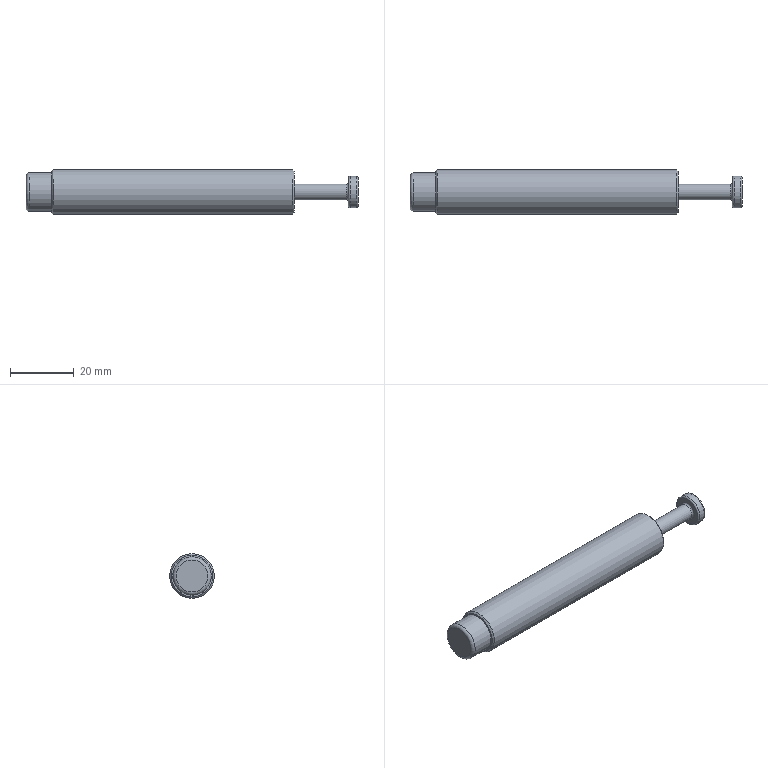Part | STEP file | Tube feed_id454_x_t | 1 solid | 15 faces | box 104 x 14 x 14 mm | volume 13153 mm3 | plane 5 | cylinder 4 | torus 4 | cone 2 | commonest cylinder face diameters 5 x1 10 x1 12 x1 14 x1
STEP:
#1=CARTESIAN_POINT('',(0.,0.,0.));
#2=DIRECTION('',(0.,0.,1.));
#3=DIRECTION('',(1.,0.,0.));
#4=AXIS2_PLACEMENT_3D('',#1,#2,#3);
#5=CARTESIAN_POINT('',(-13.,376.936,-66.));
#6=VERTEX_POINT('',#5);
#7=CARTESIAN_POINT('',(-13.,376.936,-72.));
#8=DIRECTION('',(1.,0.,0.));
#9=DIRECTION('',(0.,0.,1.));
#10=AXIS2_PLACEMENT_3D('',#7,#8,#9);
#11=CIRCLE('',#10,6.);
#12=CARTESIAN_POINT('',(-14.,376.936,-72.));
#13=DIRECTION('',(1.,0.,0.));
#14=DIRECTION('',(0.,0.,-1.));
#15=AXIS2_PLACEMENT_3D('',#12,#13,#14);
#16=CYLINDRICAL_SURFACE('',#15,6.);
#17=CARTESIAN_POINT('',(3.142,1.));
#18=DIRECTION('',(1.,0.));
#19=VECTOR('',#18,1.);
#20=LINE('',#17,#19);
#21=(GEOMETRIC_REPRESENTATION_CONTEXT(2)PARAMETRIC_REPRESENTATION_CONTEXT()REPRESENTATION_CONTEXT('',''));
#22=DEFINITIONAL_REPRESENTATION('',(#20),#21);
#23=PCURVE('',#16,#22);
#24=CARTESIAN_POINT('',(-13.,376.936,-72.));
#25=DIRECTION('',(-1.,0.,0.));
#26=DIRECTION('',(0.,0.,1.));
#27=AXIS2_PLACEMENT_3D('',#24,#25,#26);
#28=TOROIDAL_SURFACE('',#27,5.,1.);
#29=CARTESIAN_POINT('',(6.283,6.283));
#30=DIRECTION('',(-1.,0.));
#31=VECTOR('',#30,1.);
#32=LINE('',#29,#31);
#33=(GEOMETRIC_REPRESENTATION_CONTEXT(2)PARAMETRIC_REPRESENTATION_CONTEXT()REPRESENTATION_CONTEXT('',''));
#34=DEFINITIONAL_REPRESENTATION('',(#32),#33);
#35=PCURVE('',#28,#34);
#36=SURFACE_CURVE('',#11,(#23,#35),.PCURVE_S1.);
#37=EDGE_CURVE('',#6,#6,#36,.T.);
#38=ORIENTED_EDGE('',*,*,#37,.T.);
#39=CARTESIAN_POINT('',(-6.,376.936,-66.));
#40=VERTEX_POINT('',#39);
#41=CARTESIAN_POINT('',(-13.,376.936,-66.));
#42=CARTESIAN_POINT('',(-6.,376.936,-66.));
#43=B_SPLINE_CURVE_WITH_KNOTS('',1,(#41,#42),.UNSPECIFIED.,.F.,.F.,(2,2),(1.,8.),.PIECEWISE_BEZIER_KNOTS.);
#44=CARTESIAN_POINT('',(9.425,0.));
#45=DIRECTION('',(0.,1.));
#46=VECTOR('',#45,1.);
#47=LINE('',#44,#46);
#48=(GEOMETRIC_REPRESENTATION_CONTEXT(2)PARAMETRIC_REPRESENTATION_CONTEXT()REPRESENTATION_CONTEXT('',''));
#49=DEFINITIONAL_REPRESENTATION('',(#47),#48);
#50=PCURVE('',#16,#49);
#51=CARTESIAN_POINT('',(3.142,0.));
#52=DIRECTION('',(0.,1.));
#53=VECTOR('',#52,1.);
#54=LINE('',#51,#53);
#55=(GEOMETRIC_REPRESENTATION_CONTEXT(2)PARAMETRIC_REPRESENTATION_CONTEXT()REPRESENTATION_CONTEXT('',''));
#56=DEFINITIONAL_REPRESENTATION('',(#54),#55);
#57=PCURVE('',#16,#56);
#58=SEAM_CURVE('',#43,(#50,#57),.PCURVE_S1.);
#59=EDGE_CURVE('',#6,#40,#58,.T.);
#60=ORIENTED_EDGE('',*,*,#59,.T.);
#61=CARTESIAN_POINT('',(-6.,376.936,-72.));
#62=DIRECTION('',(-1.,0.,0.));
#63=DIRECTION('',(0.,0.,1.));
#64=AXIS2_PLACEMENT_3D('',#61,#62,#63);
#65=CIRCLE('',#64,6.);
#66=CARTESIAN_POINT('',(9.425,8.));
#67=DIRECTION('',(-1.,0.));
#68=VECTOR('',#67,1.);
#69=LINE('',#66,#68);
#70=(GEOMETRIC_REPRESENTATION_CONTEXT(2)PARAMETRIC_REPRESENTATION_CONTEXT()REPRESENTATION_CONTEXT('',''));
#71=DEFINITIONAL_REPRESENTATION('',(#69),#70);
#72=PCURVE('',#16,#71);
#73=CARTESIAN_POINT('',(-6.,376.936,-72.));
#74=DIRECTION('',(-1.,0.,0.));
#75=DIRECTION('',(0.,0.,1.));
#76=AXIS2_PLACEMENT_3D('',#73,#74,#75);
#77=PLANE('',#76);
#78=CARTESIAN_POINT('',(0.,0.));
#79=DIRECTION('',(1.,0.));
#80=AXIS2_PLACEMENT_2D('',#78,#79);
#81=CIRCLE('',#80,6.);
#82=(GEOMETRIC_REPRESENTATION_CONTEXT(2)PARAMETRIC_REPRESENTATION_CONTEXT()REPRESENTATION_CONTEXT('',''));
#83=DEFINITIONAL_REPRESENTATION('',(#81),#82);
#84=PCURVE('',#77,#83);
#85=SURFACE_CURVE('',#65,(#72,#84),.PCURVE_S1.);
#86=EDGE_CURVE('',#40,#40,#85,.T.);
#87=ORIENTED_EDGE('',*,*,#86,.T.);
#88=ORIENTED_EDGE('',*,*,#59,.F.);
#89=EDGE_LOOP('',(#38,#60,#87,#88));
#90=FACE_BOUND('',#89,.T.);
#91=ADVANCED_FACE('',(#90),#16,.T.);
#92=CARTESIAN_POINT('',(-14.,376.936,-67.));
#93=VERTEX_POINT('',#92);
#94=CARTESIAN_POINT('',(-14.,376.936,-72.));
#95=DIRECTION('',(-1.,0.,0.));
#96=DIRECTION('',(0.,0.,1.));
#97=AXIS2_PLACEMENT_3D('',#94,#95,#96);
#98=CIRCLE('',#97,5.);
#99=CARTESIAN_POINT('',(-14.,376.936,-72.));
#100=DIRECTION('',(-1.,0.,0.));
#101=DIRECTION('',(0.,0.,1.));
#102=AXIS2_PLACEMENT_3D('',#99,#100,#101);
#103=PLANE('',#102);
#104=CARTESIAN_POINT('',(0.,0.));
#105=DIRECTION('',(1.,0.));
#106=AXIS2_PLACEMENT_2D('',#104,#105);
#107=CIRCLE('',#106,5.);
#108=(GEOMETRIC_REPRESENTATION_CONTEXT(2)PARAMETRIC_REPRESENTATION_CONTEXT()REPRESENTATION_CONTEXT('',''));
#109=DEFINITIONAL_REPRESENTATION('',(#107),#108);
#110=PCURVE('',#103,#109);
#111=CARTESIAN_POINT('',(0.,7.854));
#112=DIRECTION('',(1.,0.));
#113=VECTOR('',#112,1.);
#114=LINE('',#111,#113);
#115=(GEOMETRIC_REPRESENTATION_CONTEXT(2)PARAMETRIC_REPRESENTATION_CONTEXT()REPRESENTATION_CONTEXT('',''));
#116=DEFINITIONAL_REPRESENTATION('',(#114),#115);
#117=PCURVE('',#28,#116);
#118=SURFACE_CURVE('',#98,(#110,#117),.PCURVE_S1.);
#119=EDGE_CURVE('',#93,#93,#118,.T.);
#120=ORIENTED_EDGE('',*,*,#119,.T.);
#121=EDGE_LOOP('',(#120));
#122=FACE_BOUND('',#121,.T.);
#123=ADVANCED_FACE('',(#122),#103,.T.);
#124=CARTESIAN_POINT('',(-6.,376.936,-65.5));
#125=VERTEX_POINT('',#124);
#126=CARTESIAN_POINT('',(-6.,376.936,-72.));
#127=DIRECTION('',(-1.,0.,0.));
#128=DIRECTION('',(0.,0.,1.));
#129=AXIS2_PLACEMENT_3D('',#126,#127,#128);
#130=CIRCLE('',#129,6.5);
#131=CARTESIAN_POINT('',(0.,0.));
#132=DIRECTION('',(1.,0.));
#133=AXIS2_PLACEMENT_2D('',#131,#132);
#134=CIRCLE('',#133,6.5);
#135=(GEOMETRIC_REPRESENTATION_CONTEXT(2)PARAMETRIC_REPRESENTATION_CONTEXT()REPRESENTATION_CONTEXT('',''));
#136=DEFINITIONAL_REPRESENTATION('',(#134),#135);
#137=PCURVE('',#77,#136);
#138=CARTESIAN_POINT('',(-5.5,376.936,-72.));
#139=DIRECTION('',(1.,0.,0.));
#140=DIRECTION('',(0.,0.,-1.));
#141=AXIS2_PLACEMENT_3D('',#138,#139,#140);
#142=CONICAL_SURFACE('',#141,7.,0.7854);
#143=CARTESIAN_POINT('',(9.425,-0.5));
#144=DIRECTION('',(-1.,0.));
#145=VECTOR('',#144,1.);
#146=LINE('',#143,#145);
#147=(GEOMETRIC_REPRESENTATION_CONTEXT(2)PARAMETRIC_REPRESENTATION_CONTEXT()REPRESENTATION_CONTEXT('',''));
#148=DEFINITIONAL_REPRESENTATION('',(#146),#147);
#149=PCURVE('',#142,#148);
#150=SURFACE_CURVE('',#130,(#137,#149),.PCURVE_S1.);
#151=EDGE_CURVE('',#125,#125,#150,.T.);
#152=ORIENTED_EDGE('',*,*,#151,.T.);
#153=EDGE_LOOP('',(#152));
#154=FACE_BOUND('',#153,.T.);
#155=ORIENTED_EDGE('',*,*,#86,.F.);
#156=EDGE_LOOP('',(#155));
#157=FACE_BOUND('',#156,.T.);
#158=ADVANCED_FACE('',(#154,#157),#77,.T.);
#159=CARTESIAN_POINT('',(70.,376.936,-74.5));
#160=VERTEX_POINT('',#159);
#161=CARTESIAN_POINT('',(70.,376.936,-72.));
#162=DIRECTION('',(1.,0.,0.));
#163=DIRECTION('',(0.,0.,-1.));
#164=AXIS2_PLACEMENT_3D('',#161,#162,#163);
#165=CIRCLE('',#164,2.5);
#166=CARTESIAN_POINT('',(70.,376.936,-72.));
#167=DIRECTION('',(-1.,0.,0.));
#168=DIRECTION('',(0.,0.,1.));
#169=AXIS2_PLACEMENT_3D('',#166,#167,#168);
#170=PLANE('',#169);
#171=CARTESIAN_POINT('',(-2.5,0.));
#172=CARTESIAN_POINT('',(-2.5,4.33));
#173=CARTESIAN_POINT('',(1.25,2.165));
#174=CARTESIAN_POINT('',(5.,0.));
#175=CARTESIAN_POINT('',(1.25,-2.165));
#176=CARTESIAN_POINT('',(-2.5,-4.33));
#177=CARTESIAN_POINT('',(-2.5,0.));
#178=(BOUNDED_CURVE()B_SPLINE_CURVE(2,(#171,#172,#173,#174,#175,#176,#177),.UNSPECIFIED.,.T.,.F.)B_SPLINE_CURVE_WITH_KNOTS((1,2,2,2,2,1),(-2.094,0.,2.094,4.189,6.283,8.378),.UNSPECIFIED.)CURVE()GEOMETRIC_REPRESENTATION_ITEM()RATIONAL_B_SPLINE_CURVE((1.,0.5,1.,0.5,1.,0.5,1.))REPRESENTATION_ITEM(''));
#179=(GEOMETRIC_REPRESENTATION_CONTEXT(2)PARAMETRIC_REPRESENTATION_CONTEXT()REPRESENTATION_CONTEXT('',''));
#180=DEFINITIONAL_REPRESENTATION('',(#178),#179);
#181=PCURVE('',#170,#180);
#182=CARTESIAN_POINT('',(90.,376.936,-72.));
#183=DIRECTION('',(-1.,0.,0.));
#184=DIRECTION('',(0.,0.,1.));
#185=AXIS2_PLACEMENT_3D('',#182,#183,#184);
#186=CYLINDRICAL_SURFACE('',#185,2.5);
#187=CARTESIAN_POINT('',(9.425,20.));
#188=DIRECTION('',(-1.,0.));
#189=VECTOR('',#188,1.);
#190=LINE('',#187,#189);
#191=(GEOMETRIC_REPRESENTATION_CONTEXT(2)PARAMETRIC_REPRESENTATION_CONTEXT()REPRESENTATION_CONTEXT('',''));
#192=DEFINITIONAL_REPRESENTATION('',(#190),#191);
#193=PCURVE('',#186,#192);
#194=SURFACE_CURVE('',#165,(#181,#193),.PCURVE_S1.);
#195=EDGE_CURVE('',#160,#160,#194,.T.);
#196=ORIENTED_EDGE('',*,*,#195,.F.);
#197=EDGE_LOOP('',(#196));
#198=FACE_BOUND('',#197,.T.);
#199=CARTESIAN_POINT('',(70.,376.936,-65.5));
#200=VERTEX_POINT('',#199);
#201=CARTESIAN_POINT('',(70.,376.936,-72.));
#202=DIRECTION('',(1.,0.,0.));
#203=DIRECTION('',(0.,0.,1.));
#204=AXIS2_PLACEMENT_3D('',#201,#202,#203);
#205=CIRCLE('',#204,6.5);
#206=CARTESIAN_POINT('',(6.5,0.));
#207=CARTESIAN_POINT('',(6.5,-11.258));
#208=CARTESIAN_POINT('',(-3.25,-5.629));
#209=CARTESIAN_POINT('',(-13.,0.));
#210=CARTESIAN_POINT('',(-3.25,5.629));
#211=CARTESIAN_POINT('',(6.5,11.258));
#212=CARTESIAN_POINT('',(6.5,0.));
#213=(BOUNDED_CURVE()B_SPLINE_CURVE(2,(#206,#207,#208,#209,#210,#211,#212),.UNSPECIFIED.,.T.,.F.)B_SPLINE_CURVE_WITH_KNOTS((1,2,2,2,2,1),(-2.094,0.,2.094,4.189,6.283,8.378),.UNSPECIFIED.)CURVE()GEOMETRIC_REPRESENTATION_ITEM()RATIONAL_B_SPLINE_CURVE((1.,0.5,1.,0.5,1.,0.5,1.))REPRESENTATION_ITEM(''));
#214=(GEOMETRIC_REPRESENTATION_CONTEXT(2)PARAMETRIC_REPRESENTATION_CONTEXT()REPRESENTATION_CONTEXT('',''));
#215=DEFINITIONAL_REPRESENTATION('',(#213),#214);
#216=PCURVE('',#170,#215);
#217=CARTESIAN_POINT('',(69.5,376.936,-72.));
#218=DIRECTION('',(-1.,0.,0.));
#219=DIRECTION('',(0.,0.,1.));
#220=AXIS2_PLACEMENT_3D('',#217,#218,#219);
#221=CONICAL_SURFACE('',#220,7.,0.7854);
#222=CARTESIAN_POINT('',(6.283,-0.5));
#223=DIRECTION('',(-1.,0.));
#224=VECTOR('',#223,1.);
#225=LINE('',#222,#224);
#226=(GEOMETRIC_REPRESENTATION_CONTEXT(2)PARAMETRIC_REPRESENTATION_CONTEXT()REPRESENTATION_CONTEXT('',''));
#227=DEFINITIONAL_REPRESENTATION('',(#225),#226);
#228=PCURVE('',#221,#227);
#229=SURFACE_CURVE('',#205,(#216,#228),.PCURVE_S1.);
#230=EDGE_CURVE('',#200,#200,#229,.T.);
#231=ORIENTED_EDGE('',*,*,#230,.T.);
#232=EDGE_LOOP('',(#231));
#233=FACE_BOUND('',#232,.T.);
#234=ADVANCED_FACE('',(#198,#233),#170,.F.);
#235=CARTESIAN_POINT('',(-5.5,376.936,-65.));
#236=VERTEX_POINT('',#235);
#237=CARTESIAN_POINT('',(-5.5,376.936,-72.));
#238=DIRECTION('',(1.,0.,0.));
#239=DIRECTION('',(0.,0.,1.));
#240=AXIS2_PLACEMENT_3D('',#237,#238,#239);
#241=CIRCLE('',#240,7.);
#242=CARTESIAN_POINT('',(-6.,376.936,-72.));
#243=DIRECTION('',(1.,0.,0.));
#244=DIRECTION('',(0.,0.,-1.));
#245=AXIS2_PLACEMENT_3D('',#242,#243,#244);
#246=CYLINDRICAL_SURFACE('',#245,7.);
#247=CARTESIAN_POINT('',(3.142,0.5));
#248=DIRECTION('',(1.,0.));
#249=VECTOR('',#248,1.);
#250=LINE('',#247,#249);
#251=(GEOMETRIC_REPRESENTATION_CONTEXT(2)PARAMETRIC_REPRESENTATION_CONTEXT()REPRESENTATION_CONTEXT('',''));
#252=DEFINITIONAL_REPRESENTATION('',(#250),#251);
#253=PCURVE('',#246,#252);
#254=CARTESIAN_POINT('',(3.142,0.));
#255=DIRECTION('',(1.,0.));
#256=VECTOR('',#255,1.);
#257=LINE('',#254,#256);
#258=(GEOMETRIC_REPRESENTATION_CONTEXT(2)PARAMETRIC_REPRESENTATION_CONTEXT()REPRESENTATION_CONTEXT('',''));
#259=DEFINITIONAL_REPRESENTATION('',(#257),#258);
#260=PCURVE('',#142,#259);
#261=SURFACE_CURVE('',#241,(#253,#260),.PCURVE_S1.);
#262=EDGE_CURVE('',#236,#236,#261,.T.);
#263=ORIENTED_EDGE('',*,*,#262,.T.);
#264=CARTESIAN_POINT('',(69.5,376.936,-65.));
#265=VERTEX_POINT('',#264);
#266=CARTESIAN_POINT('',(-5.5,376.936,-65.));
#267=CARTESIAN_POINT('',(69.5,376.936,-65.));
#268=B_SPLINE_CURVE_WITH_KNOTS('',1,(#266,#267),.UNSPECIFIED.,.F.,.F.,(2,2),(0.5,75.5),.PIECEWISE_BEZIER_KNOTS.);
#269=CARTESIAN_POINT('',(9.425,0.));
#270=DIRECTION('',(0.,1.));
#271=VECTOR('',#270,1.);
#272=LINE('',#269,#271);
#273=(GEOMETRIC_REPRESENTATION_CONTEXT(2)PARAMETRIC_REPRESENTATION_CONTEXT()REPRESENTATION_CONTEXT('',''));
#274=DEFINITIONAL_REPRESENTATION('',(#272),#273);
#275=PCURVE('',#246,#274);
#276=CARTESIAN_POINT('',(3.142,0.));
#277=DIRECTION('',(0.,1.));
#278=VECTOR('',#277,1.);
#279=LINE('',#276,#278);
#280=(GEOMETRIC_REPRESENTATION_CONTEXT(2)PARAMETRIC_REPRESENTATION_CONTEXT()REPRESENTATION_CONTEXT('',''));
#281=DEFINITIONAL_REPRESENTATION('',(#279),#280);
#282=PCURVE('',#246,#281);
#283=SEAM_CURVE('',#268,(#275,#282),.PCURVE_S1.);
#284=EDGE_CURVE('',#236,#265,#283,.T.);
#285=ORIENTED_EDGE('',*,*,#284,.T.);
#286=CARTESIAN_POINT('',(69.5,376.936,-72.));
#287=DIRECTION('',(-1.,0.,0.));
#288=DIRECTION('',(0.,0.,1.));
#289=AXIS2_PLACEMENT_3D('',#286,#287,#288);
#290=CIRCLE('',#289,7.);
#291=CARTESIAN_POINT('',(9.425,75.5));
#292=DIRECTION('',(-1.,0.));
#293=VECTOR('',#292,1.);
#294=LINE('',#291,#293);
#295=(GEOMETRIC_REPRESENTATION_CONTEXT(2)PARAMETRIC_REPRESENTATION_CONTEXT()REPRESENTATION_CONTEXT('',''));
#296=DEFINITIONAL_REPRESENTATION('',(#294),#295);
#297=PCURVE('',#246,#296);
#298=CARTESIAN_POINT('',(0.,0.));
#299=DIRECTION('',(1.,0.));
#300=VECTOR('',#299,1.);
#301=LINE('',#298,#300);
#302=(GEOMETRIC_REPRESENTATION_CONTEXT(2)PARAMETRIC_REPRESENTATION_CONTEXT()REPRESENTATION_CONTEXT('',''));
#303=DEFINITIONAL_REPRESENTATION('',(#301),#302);
#304=PCURVE('',#221,#303);
#305=SURFACE_CURVE('',#290,(#297,#304),.PCURVE_S1.);
#306=EDGE_CURVE('',#265,#265,#305,.T.);
#307=ORIENTED_EDGE('',*,*,#306,.T.);
#308=ORIENTED_EDGE('',*,*,#284,.F.);
#309=EDGE_LOOP('',(#263,#285,#307,#308));
#310=FACE_BOUND('',#309,.T.);
#311=ADVANCED_FACE('',(#310),#246,.T.);
#312=ORIENTED_EDGE('',*,*,#230,.F.);
#313=CARTESIAN_POINT('',(70.,376.936,-65.5));
#314=CARTESIAN_POINT('',(69.5,376.936,-65.));
#315=B_SPLINE_CURVE_WITH_KNOTS('',1,(#313,#314),.UNSPECIFIED.,.F.,.F.,(2,2),(-0.7071,0.),.PIECEWISE_BEZIER_KNOTS.);
#316=CARTESIAN_POINT('',(6.283,0.));
#317=DIRECTION('',(0.,1.));
#318=VECTOR('',#317,1.);
#319=LINE('',#316,#318);
#320=(GEOMETRIC_REPRESENTATION_CONTEXT(2)PARAMETRIC_REPRESENTATION_CONTEXT()REPRESENTATION_CONTEXT('',''));
#321=DEFINITIONAL_REPRESENTATION('',(#319),#320);
#322=PCURVE('',#221,#321);
#323=CARTESIAN_POINT('',(0.,0.));
#324=DIRECTION('',(0.,1.));
#325=VECTOR('',#324,1.);
#326=LINE('',#323,#325);
#327=(GEOMETRIC_REPRESENTATION_CONTEXT(2)PARAMETRIC_REPRESENTATION_CONTEXT()REPRESENTATION_CONTEXT('',''));
#328=DEFINITIONAL_REPRESENTATION('',(#326),#327);
#329=PCURVE('',#221,#328);
#330=SEAM_CURVE('',#315,(#322,#329),.PCURVE_S1.);
#331=EDGE_CURVE('',#200,#265,#330,.T.);
#332=ORIENTED_EDGE('',*,*,#331,.T.);
#333=ORIENTED_EDGE('',*,*,#306,.F.);
#334=ORIENTED_EDGE('',*,*,#331,.F.);
#335=EDGE_LOOP('',(#312,#332,#333,#334));
#336=FACE_BOUND('',#335,.T.);
#337=ADVANCED_FACE('',(#336),#221,.T.);
#338=ORIENTED_EDGE('',*,*,#151,.F.);
#339=CARTESIAN_POINT('',(-6.,376.936,-65.5));
#340=CARTESIAN_POINT('',(-5.5,376.936,-65.));
#341=B_SPLINE_CURVE_WITH_KNOTS('',1,(#339,#340),.UNSPECIFIED.,.F.,.F.,(2,2),(-0.7071,0.),.PIECEWISE_BEZIER_KNOTS.);
#342=CARTESIAN_POINT('',(9.425,0.));
#343=DIRECTION('',(0.,1.));
#344=VECTOR('',#343,1.);
#345=LINE('',#342,#344);
#346=(GEOMETRIC_REPRESENTATION_CONTEXT(2)PARAMETRIC_REPRESENTATION_CONTEXT()REPRESENTATION_CONTEXT('',''));
#347=DEFINITIONAL_REPRESENTATION('',(#345),#346);
#348=PCURVE('',#142,#347);
#349=CARTESIAN_POINT('',(3.142,0.));
#350=DIRECTION('',(0.,1.));
#351=VECTOR('',#350,1.);
#352=LINE('',#349,#351);
#353=(GEOMETRIC_REPRESENTATION_CONTEXT(2)PARAMETRIC_REPRESENTATION_CONTEXT()REPRESENTATION_CONTEXT('',''));
#354=DEFINITIONAL_REPRESENTATION('',(#352),#353);
#355=PCURVE('',#142,#354);
#356=SEAM_CURVE('',#341,(#348,#355),.PCURVE_S1.);
#357=EDGE_CURVE('',#125,#236,#356,.T.);
#358=ORIENTED_EDGE('',*,*,#357,.T.);
#359=ORIENTED_EDGE('',*,*,#262,.F.);
#360=ORIENTED_EDGE('',*,*,#357,.F.);
#361=EDGE_LOOP('',(#338,#358,#359,#360));
#362=FACE_BOUND('',#361,.T.);
#363=ADVANCED_FACE('',(#362),#142,.T.);
#364=ORIENTED_EDGE('',*,*,#37,.F.);
#365=CARTESIAN_POINT('',(-13.,376.936,-66.));
#366=CARTESIAN_POINT('',(-13.267,376.936,-66.));
#367=CARTESIAN_POINT('',(-13.528,376.936,-66.085));
#368=CARTESIAN_POINT('',(-13.752,376.936,-66.248));
#369=CARTESIAN_POINT('',(-13.915,376.936,-66.472));
#370=CARTESIAN_POINT('',(-14.,376.936,-66.733));
#371=CARTESIAN_POINT('',(-14.,376.936,-67.));
#372=(BOUNDED_CURVE()B_SPLINE_CURVE(6,(#365,#366,#367,#368,#369,#370,#371),.UNSPECIFIED.,.F.,.F.)B_SPLINE_CURVE_WITH_KNOTS((7,7),(0.,1.571),.PIECEWISE_BEZIER_KNOTS.)CURVE()GEOMETRIC_REPRESENTATION_ITEM()RATIONAL_B_SPLINE_CURVE((1.031,1.01,0.9979,0.994,0.9979,1.01,1.031))REPRESENTATION_ITEM(''));
#373=CARTESIAN_POINT('',(6.283,6.283));
#374=DIRECTION('',(0.,1.));
#375=VECTOR('',#374,1.);
#376=LINE('',#373,#375);
#377=(GEOMETRIC_REPRESENTATION_CONTEXT(2)PARAMETRIC_REPRESENTATION_CONTEXT()REPRESENTATION_CONTEXT('',''));
#378=DEFINITIONAL_REPRESENTATION('',(#376),#377);
#379=PCURVE('',#28,#378);
#380=CARTESIAN_POINT('',(0.,6.283));
#381=DIRECTION('',(0.,1.));
#382=VECTOR('',#381,1.);
#383=LINE('',#380,#382);
#384=(GEOMETRIC_REPRESENTATION_CONTEXT(2)PARAMETRIC_REPRESENTATION_CONTEXT()REPRESENTATION_CONTEXT('',''));
#385=DEFINITIONAL_REPRESENTATION('',(#383),#384);
#386=PCURVE('',#28,#385);
#387=SEAM_CURVE('',#372,(#379,#386),.PCURVE_S1.);
#388=EDGE_CURVE('',#6,#93,#387,.T.);
#389=ORIENTED_EDGE('',*,*,#388,.T.);
#390=ORIENTED_EDGE('',*,*,#119,.F.);
#391=ORIENTED_EDGE('',*,*,#388,.F.);
#392=EDGE_LOOP('',(#364,#389,#390,#391));
#393=FACE_BOUND('',#392,.T.);
#394=ADVANCED_FACE('',(#393),#28,.T.);
#395=CARTESIAN_POINT('',(86.5,376.936,-74.5));
#396=VERTEX_POINT('',#395);
#397=CARTESIAN_POINT('',(86.5,376.936,-72.));
#398=DIRECTION('',(-1.,0.,0.));
#399=DIRECTION('',(0.,0.,-1.));
#400=AXIS2_PLACEMENT_3D('',#397,#398,#399);
#401=CIRCLE('',#400,2.5);
#402=CARTESIAN_POINT('',(3.142,3.5));
#403=DIRECTION('',(1.,0.));
#404=VECTOR('',#403,1.);
#405=LINE('',#402,#404);
#406=(GEOMETRIC_REPRESENTATION_CONTEXT(2)PARAMETRIC_REPRESENTATION_CONTEXT()REPRESENTATION_CONTEXT('',''));
#407=DEFINITIONAL_REPRESENTATION('',(#405),#406);
#408=PCURVE('',#186,#407);
#409=CARTESIAN_POINT('',(86.5,376.936,-72.));
#410=DIRECTION('',(1.,0.,0.));
#411=DIRECTION('',(0.,0.,-1.));
#412=AXIS2_PLACEMENT_3D('',#409,#410,#411);
#413=TOROIDAL_SURFACE('',#412,3.,0.5);
#414=CARTESIAN_POINT('',(6.283,9.425));
#415=DIRECTION('',(-1.,0.));
#416=VECTOR('',#415,1.);
#417=LINE('',#414,#416);
#418=(GEOMETRIC_REPRESENTATION_CONTEXT(2)PARAMETRIC_REPRESENTATION_CONTEXT()REPRESENTATION_CONTEXT('',''));
#419=DEFINITIONAL_REPRESENTATION('',(#417),#418);
#420=PCURVE('',#413,#419);
#421=SURFACE_CURVE('',#401,(#408,#420),.PCURVE_S1.);
#422=EDGE_CURVE('',#396,#396,#421,.T.);
#423=ORIENTED_EDGE('',*,*,#422,.T.);
#424=CARTESIAN_POINT('',(86.5,376.936,-74.5));
#425=CARTESIAN_POINT('',(70.,376.936,-74.5));
#426=B_SPLINE_CURVE_WITH_KNOTS('',1,(#424,#425),.UNSPECIFIED.,.F.,.F.,(2,2),(3.5,20.),.PIECEWISE_BEZIER_KNOTS.);
#427=CARTESIAN_POINT('',(9.425,0.));
#428=DIRECTION('',(0.,1.));
#429=VECTOR('',#428,1.);
#430=LINE('',#427,#429);
#431=(GEOMETRIC_REPRESENTATION_CONTEXT(2)PARAMETRIC_REPRESENTATION_CONTEXT()REPRESENTATION_CONTEXT('',''));
#432=DEFINITIONAL_REPRESENTATION('',(#430),#431);
#433=PCURVE('',#186,#432);
#434=CARTESIAN_POINT('',(3.142,0.));
#435=DIRECTION('',(0.,1.));
#436=VECTOR('',#435,1.);
#437=LINE('',#434,#436);
#438=(GEOMETRIC_REPRESENTATION_CONTEXT(2)PARAMETRIC_REPRESENTATION_CONTEXT()REPRESENTATION_CONTEXT('',''));
#439=DEFINITIONAL_REPRESENTATION('',(#437),#438);
#440=PCURVE('',#186,#439);
#441=SEAM_CURVE('',#426,(#433,#440),.PCURVE_S1.);
#442=EDGE_CURVE('',#396,#160,#441,.T.);
#443=ORIENTED_EDGE('',*,*,#442,.T.);
#444=ORIENTED_EDGE('',*,*,#195,.T.);
#445=ORIENTED_EDGE('',*,*,#442,.F.);
#446=EDGE_LOOP('',(#423,#443,#444,#445));
#447=FACE_BOUND('',#446,.T.);
#448=ADVANCED_FACE('',(#447),#186,.T.);
#449=CARTESIAN_POINT('',(87.5,376.936,-77.));
#450=VERTEX_POINT('',#449);
#451=CARTESIAN_POINT('',(87.5,376.936,-72.));
#452=DIRECTION('',(1.,0.,0.));
#453=DIRECTION('',(0.,0.,-1.));
#454=AXIS2_PLACEMENT_3D('',#451,#452,#453);
#455=CIRCLE('',#454,5.);
#456=CARTESIAN_POINT('',(87.,376.936,-72.));
#457=DIRECTION('',(1.,0.,0.));
#458=DIRECTION('',(0.,0.,-1.));
#459=AXIS2_PLACEMENT_3D('',#456,#457,#458);
#460=CYLINDRICAL_SURFACE('',#459,5.);
#461=CARTESIAN_POINT('',(0.,0.5));
#462=DIRECTION('',(1.,0.));
#463=VECTOR('',#462,1.);
#464=LINE('',#461,#463);
#465=(GEOMETRIC_REPRESENTATION_CONTEXT(2)PARAMETRIC_REPRESENTATION_CONTEXT()REPRESENTATION_CONTEXT('',''));
#466=DEFINITIONAL_REPRESENTATION('',(#464),#465);
#467=PCURVE('',#460,#466);
#468=CARTESIAN_POINT('',(87.5,376.936,-72.));
#469=DIRECTION('',(1.,0.,0.));
#470=DIRECTION('',(0.,0.,-1.));
#471=AXIS2_PLACEMENT_3D('',#468,#469,#470);
#472=TOROIDAL_SURFACE('',#471,4.5,0.5);
#473=CARTESIAN_POINT('',(0.,6.283));
#474=DIRECTION('',(1.,0.));
#475=VECTOR('',#474,1.);
#476=LINE('',#473,#475);
#477=(GEOMETRIC_REPRESENTATION_CONTEXT(2)PARAMETRIC_REPRESENTATION_CONTEXT()REPRESENTATION_CONTEXT('',''));
#478=DEFINITIONAL_REPRESENTATION('',(#476),#477);
#479=PCURVE('',#472,#478);
#480=SURFACE_CURVE('',#455,(#467,#479),.PCURVE_S1.);
#481=EDGE_CURVE('',#450,#450,#480,.T.);
#482=ORIENTED_EDGE('',*,*,#481,.T.);
#483=CARTESIAN_POINT('',(89.5,376.936,-77.));
#484=VERTEX_POINT('',#483);
#485=CARTESIAN_POINT('',(87.5,376.936,-77.));
#486=CARTESIAN_POINT('',(89.5,376.936,-77.));
#487=B_SPLINE_CURVE_WITH_KNOTS('',1,(#485,#486),.UNSPECIFIED.,.F.,.F.,(2,2),(0.5,2.5),.PIECEWISE_BEZIER_KNOTS.);
#488=CARTESIAN_POINT('',(6.283,0.));
#489=DIRECTION('',(0.,1.));
#490=VECTOR('',#489,1.);
#491=LINE('',#488,#490);
#492=(GEOMETRIC_REPRESENTATION_CONTEXT(2)PARAMETRIC_REPRESENTATION_CONTEXT()REPRESENTATION_CONTEXT('',''));
#493=DEFINITIONAL_REPRESENTATION('',(#491),#492);
#494=PCURVE('',#460,#493);
#495=CARTESIAN_POINT('',(0.,0.));
#496=DIRECTION('',(0.,1.));
#497=VECTOR('',#496,1.);
#498=LINE('',#495,#497);
#499=(GEOMETRIC_REPRESENTATION_CONTEXT(2)PARAMETRIC_REPRESENTATION_CONTEXT()REPRESENTATION_CONTEXT('',''));
#500=DEFINITIONAL_REPRESENTATION('',(#498),#499);
#501=PCURVE('',#460,#500);
#502=SEAM_CURVE('',#487,(#494,#501),.PCURVE_S1.);
#503=EDGE_CURVE('',#450,#484,#502,.T.);
#504=ORIENTED_EDGE('',*,*,#503,.T.);
#505=CARTESIAN_POINT('',(89.5,376.936,-72.));
#506=DIRECTION('',(-1.,0.,0.));
#507=DIRECTION('',(0.,0.,-1.));
#508=AXIS2_PLACEMENT_3D('',#505,#506,#507);
#509=CIRCLE('',#508,5.);
#510=CARTESIAN_POINT('',(6.283,2.5));
#511=DIRECTION('',(-1.,0.));
#512=VECTOR('',#511,1.);
#513=LINE('',#510,#512);
#514=(GEOMETRIC_REPRESENTATION_CONTEXT(2)PARAMETRIC_REPRESENTATION_CONTEXT()REPRESENTATION_CONTEXT('',''));
#515=DEFINITIONAL_REPRESENTATION('',(#513),#514);
#516=PCURVE('',#460,#515);
#517=CARTESIAN_POINT('',(89.5,376.936,-72.));
#518=DIRECTION('',(1.,0.,0.));
#519=DIRECTION('',(0.,0.,-1.));
#520=AXIS2_PLACEMENT_3D('',#517,#518,#519);
#521=TOROIDAL_SURFACE('',#520,4.5,0.5);
#522=CARTESIAN_POINT('',(6.283,6.283));
#523=DIRECTION('',(-1.,0.));
#524=VECTOR('',#523,1.);
#525=LINE('',#522,#524);
#526=(GEOMETRIC_REPRESENTATION_CONTEXT(2)PARAMETRIC_REPRESENTATION_CONTEXT()REPRESENTATION_CONTEXT('',''));
#527=DEFINITIONAL_REPRESENTATION('',(#525),#526);
#528=PCURVE('',#521,#527);
#529=SURFACE_CURVE('',#509,(#516,#528),.PCURVE_S1.);
#530=EDGE_CURVE('',#484,#484,#529,.T.);
#531=ORIENTED_EDGE('',*,*,#530,.T.);
#532=ORIENTED_EDGE('',*,*,#503,.F.);
#533=EDGE_LOOP('',(#482,#504,#531,#532));
#534=FACE_BOUND('',#533,.T.);
#535=ADVANCED_FACE('',(#534),#460,.T.);
#536=CARTESIAN_POINT('',(87.,376.936,-75.));
#537=VERTEX_POINT('',#536);
#538=CARTESIAN_POINT('',(87.,376.936,-72.));
#539=DIRECTION('',(1.,0.,0.));
#540=DIRECTION('',(0.,0.,-1.));
#541=AXIS2_PLACEMENT_3D('',#538,#539,#540);
#542=CIRCLE('',#541,3.);
#543=CARTESIAN_POINT('',(87.,376.936,-72.));
#544=DIRECTION('',(1.,0.,0.));
#545=DIRECTION('',(0.,0.,-1.));
#546=AXIS2_PLACEMENT_3D('',#543,#544,#545);
#547=PLANE('',#546);
#548=CARTESIAN_POINT('',(0.,0.));
#549=DIRECTION('',(1.,0.));
#550=AXIS2_PLACEMENT_2D('',#548,#549);
#551=CIRCLE('',#550,3.);
#552=(GEOMETRIC_REPRESENTATION_CONTEXT(2)PARAMETRIC_REPRESENTATION_CONTEXT()REPRESENTATION_CONTEXT('',''));
#553=DEFINITIONAL_REPRESENTATION('',(#551),#552);
#554=PCURVE('',#547,#553);
#555=CARTESIAN_POINT('',(0.,7.854));
#556=DIRECTION('',(1.,0.));
#557=VECTOR('',#556,1.);
#558=LINE('',#555,#557);
#559=(GEOMETRIC_REPRESENTATION_CONTEXT(2)PARAMETRIC_REPRESENTATION_CONTEXT()REPRESENTATION_CONTEXT('',''));
#560=DEFINITIONAL_REPRESENTATION('',(#558),#559);
#561=PCURVE('',#413,#560);
#562=SURFACE_CURVE('',#542,(#554,#561),.PCURVE_S1.);
#563=EDGE_CURVE('',#537,#537,#562,.T.);
#564=ORIENTED_EDGE('',*,*,#563,.T.);
#565=EDGE_LOOP('',(#564));
#566=FACE_BOUND('',#565,.T.);
#567=CARTESIAN_POINT('',(87.,376.936,-76.5));
#568=VERTEX_POINT('',#567);
#569=CARTESIAN_POINT('',(87.,376.936,-72.));
#570=DIRECTION('',(-1.,0.,0.));
#571=DIRECTION('',(0.,0.,-1.));
#572=AXIS2_PLACEMENT_3D('',#569,#570,#571);
#573=CIRCLE('',#572,4.5);
#574=CARTESIAN_POINT('',(4.5,0.));
#575=CARTESIAN_POINT('',(4.5,-7.794));
#576=CARTESIAN_POINT('',(-2.25,-3.897));
#577=CARTESIAN_POINT('',(-9.,0.));
#578=CARTESIAN_POINT('',(-2.25,3.897));
#579=CARTESIAN_POINT('',(4.5,7.794));
#580=CARTESIAN_POINT('',(4.5,0.));
#581=(BOUNDED_CURVE()B_SPLINE_CURVE(2,(#574,#575,#576,#577,#578,#579,#580),.UNSPECIFIED.,.T.,.F.)B_SPLINE_CURVE_WITH_KNOTS((1,2,2,2,2,1),(-2.094,0.,2.094,4.189,6.283,8.378),.UNSPECIFIED.)CURVE()GEOMETRIC_REPRESENTATION_ITEM()RATIONAL_B_SPLINE_CURVE((1.,0.5,1.,0.5,1.,0.5,1.))REPRESENTATION_ITEM(''));
#582=(GEOMETRIC_REPRESENTATION_CONTEXT(2)PARAMETRIC_REPRESENTATION_CONTEXT()REPRESENTATION_CONTEXT('',''));
#583=DEFINITIONAL_REPRESENTATION('',(#581),#582);
#584=PCURVE('',#547,#583);
#585=CARTESIAN_POINT('',(6.283,4.712));
#586=DIRECTION('',(-1.,0.));
#587=VECTOR('',#586,1.);
#588=LINE('',#585,#587);
#589=(GEOMETRIC_REPRESENTATION_CONTEXT(2)PARAMETRIC_REPRESENTATION_CONTEXT()REPRESENTATION_CONTEXT('',''));
#590=DEFINITIONAL_REPRESENTATION('',(#588),#589);
#591=PCURVE('',#472,#590);
#592=SURFACE_CURVE('',#573,(#584,#591),.PCURVE_S1.);
#593=EDGE_CURVE('',#568,#568,#592,.T.);
#594=ORIENTED_EDGE('',*,*,#593,.T.);
#595=EDGE_LOOP('',(#594));
#596=FACE_BOUND('',#595,.T.);
#597=ADVANCED_FACE('',(#566,#596),#547,.F.);
#598=CARTESIAN_POINT('',(90.,376.936,-76.5));
#599=VERTEX_POINT('',#598);
#600=CARTESIAN_POINT('',(90.,376.936,-72.));
#601=DIRECTION('',(1.,0.,0.));
#602=DIRECTION('',(0.,0.,-1.));
#603=AXIS2_PLACEMENT_3D('',#600,#601,#602);
#604=CIRCLE('',#603,4.5);
#605=CARTESIAN_POINT('',(90.,376.936,-72.));
#606=DIRECTION('',(1.,0.,0.));
#607=DIRECTION('',(0.,0.,-1.));
#608=AXIS2_PLACEMENT_3D('',#605,#606,#607);
#609=PLANE('',#608);
#610=CARTESIAN_POINT('',(0.,0.));
#611=DIRECTION('',(1.,0.));
#612=AXIS2_PLACEMENT_2D('',#610,#611);
#613=CIRCLE('',#612,4.5);
#614=(GEOMETRIC_REPRESENTATION_CONTEXT(2)PARAMETRIC_REPRESENTATION_CONTEXT()REPRESENTATION_CONTEXT('',''));
#615=DEFINITIONAL_REPRESENTATION('',(#613),#614);
#616=PCURVE('',#609,#615);
#617=CARTESIAN_POINT('',(0.,7.854));
#618=DIRECTION('',(1.,0.));
#619=VECTOR('',#618,1.);
#620=LINE('',#617,#619);
#621=(GEOMETRIC_REPRESENTATION_CONTEXT(2)PARAMETRIC_REPRESENTATION_CONTEXT()REPRESENTATION_CONTEXT('',''));
#622=DEFINITIONAL_REPRESENTATION('',(#620),#621);
#623=PCURVE('',#521,#622);
#624=SURFACE_CURVE('',#604,(#616,#623),.PCURVE_S1.);
#625=EDGE_CURVE('',#599,#599,#624,.T.);
#626=ORIENTED_EDGE('',*,*,#625,.T.);
#627=EDGE_LOOP('',(#626));
#628=FACE_BOUND('',#627,.T.);
#629=ADVANCED_FACE('',(#628),#609,.T.);
#630=ORIENTED_EDGE('',*,*,#422,.T.);
#631=CARTESIAN_POINT('',(87.,376.936,-75.));
#632=CARTESIAN_POINT('',(87.,376.936,-74.866));
#633=CARTESIAN_POINT('',(86.957,376.936,-74.736));
#634=CARTESIAN_POINT('',(86.876,376.936,-74.624));
#635=CARTESIAN_POINT('',(86.764,376.936,-74.543));
#636=CARTESIAN_POINT('',(86.634,376.936,-74.5));
#637=CARTESIAN_POINT('',(86.5,376.936,-74.5));
#638=(BOUNDED_CURVE()B_SPLINE_CURVE(6,(#631,#632,#633,#634,#635,#636,#637),.UNSPECIFIED.,.F.,.F.)B_SPLINE_CURVE_WITH_KNOTS((7,7),(1.571,3.142),.PIECEWISE_BEZIER_KNOTS.)CURVE()GEOMETRIC_REPRESENTATION_ITEM()RATIONAL_B_SPLINE_CURVE((1.031,1.01,0.9979,0.994,0.9979,1.01,1.031))REPRESENTATION_ITEM(''));
#639=CARTESIAN_POINT('',(0.,6.283));
#640=DIRECTION('',(0.,1.));
#641=VECTOR('',#640,1.);
#642=LINE('',#639,#641);
#643=(GEOMETRIC_REPRESENTATION_CONTEXT(2)PARAMETRIC_REPRESENTATION_CONTEXT()REPRESENTATION_CONTEXT('',''));
#644=DEFINITIONAL_REPRESENTATION('',(#642),#643);
#645=PCURVE('',#413,#644);
#646=CARTESIAN_POINT('',(6.283,6.283));
#647=DIRECTION('',(0.,1.));
#648=VECTOR('',#647,1.);
#649=LINE('',#646,#648);
#650=(GEOMETRIC_REPRESENTATION_CONTEXT(2)PARAMETRIC_REPRESENTATION_CONTEXT()REPRESENTATION_CONTEXT('',''));
#651=DEFINITIONAL_REPRESENTATION('',(#649),#650);
#652=PCURVE('',#413,#651);
#653=SEAM_CURVE('',#638,(#645,#652),.PCURVE_S1.);
#654=EDGE_CURVE('',#537,#396,#653,.T.);
#655=ORIENTED_EDGE('',*,*,#654,.F.);
#656=ORIENTED_EDGE('',*,*,#563,.T.);
#657=ORIENTED_EDGE('',*,*,#654,.T.);
#658=EDGE_LOOP('',(#630,#655,#656,#657));
#659=FACE_BOUND('',#658,.F.);
#660=ADVANCED_FACE('',(#659),#413,.F.);
#661=ORIENTED_EDGE('',*,*,#593,.F.);
#662=CARTESIAN_POINT('',(87.,376.936,-76.5));
#663=CARTESIAN_POINT('',(87.,376.936,-76.634));
#664=CARTESIAN_POINT('',(87.043,376.936,-76.764));
#665=CARTESIAN_POINT('',(87.124,376.936,-76.876));
#666=CARTESIAN_POINT('',(87.236,376.936,-76.957));
#667=CARTESIAN_POINT('',(87.366,376.936,-77.));
#668=CARTESIAN_POINT('',(87.5,376.936,-77.));
#669=(BOUNDED_CURVE()B_SPLINE_CURVE(6,(#662,#663,#664,#665,#666,#667,#668),.UNSPECIFIED.,.F.,.F.)B_SPLINE_CURVE_WITH_KNOTS((7,7),(4.712,6.283),.PIECEWISE_BEZIER_KNOTS.)CURVE()GEOMETRIC_REPRESENTATION_ITEM()RATIONAL_B_SPLINE_CURVE((1.031,1.01,0.9979,0.994,0.9979,1.01,1.031))REPRESENTATION_ITEM(''));
#670=CARTESIAN_POINT('',(6.283,0.));
#671=DIRECTION('',(0.,1.));
#672=VECTOR('',#671,1.);
#673=LINE('',#670,#672);
#674=(GEOMETRIC_REPRESENTATION_CONTEXT(2)PARAMETRIC_REPRESENTATION_CONTEXT()REPRESENTATION_CONTEXT('',''));
#675=DEFINITIONAL_REPRESENTATION('',(#673),#674);
#676=PCURVE('',#472,#675);
#677=CARTESIAN_POINT('',(0.,0.));
#678=DIRECTION('',(0.,1.));
#679=VECTOR('',#678,1.);
#680=LINE('',#677,#679);
#681=(GEOMETRIC_REPRESENTATION_CONTEXT(2)PARAMETRIC_REPRESENTATION_CONTEXT()REPRESENTATION_CONTEXT('',''));
#682=DEFINITIONAL_REPRESENTATION('',(#680),#681);
#683=PCURVE('',#472,#682);
#684=SEAM_CURVE('',#669,(#676,#683),.PCURVE_S1.);
#685=EDGE_CURVE('',#568,#450,#684,.T.);
#686=ORIENTED_EDGE('',*,*,#685,.T.);
#687=ORIENTED_EDGE('',*,*,#481,.F.);
#688=ORIENTED_EDGE('',*,*,#685,.F.);
#689=EDGE_LOOP('',(#661,#686,#687,#688));
#690=FACE_BOUND('',#689,.T.);
#691=ADVANCED_FACE('',(#690),#472,.T.);
#692=ORIENTED_EDGE('',*,*,#530,.F.);
#693=CARTESIAN_POINT('',(89.5,376.936,-77.));
#694=CARTESIAN_POINT('',(89.634,376.936,-77.));
#695=CARTESIAN_POINT('',(89.764,376.936,-76.957));
#696=CARTESIAN_POINT('',(89.876,376.936,-76.876));
#697=CARTESIAN_POINT('',(89.957,376.936,-76.764));
#698=CARTESIAN_POINT('',(90.,376.936,-76.634));
#699=CARTESIAN_POINT('',(90.,376.936,-76.5));
#700=(BOUNDED_CURVE()B_SPLINE_CURVE(6,(#693,#694,#695,#696,#697,#698,#699),.UNSPECIFIED.,.F.,.F.)B_SPLINE_CURVE_WITH_KNOTS((7,7),(0.,1.571),.PIECEWISE_BEZIER_KNOTS.)CURVE()GEOMETRIC_REPRESENTATION_ITEM()RATIONAL_B_SPLINE_CURVE((1.031,1.01,0.9979,0.994,0.9979,1.01,1.031))REPRESENTATION_ITEM(''));
#701=CARTESIAN_POINT('',(6.283,6.283));
#702=DIRECTION('',(0.,1.));
#703=VECTOR('',#702,1.);
#704=LINE('',#701,#703);
#705=(GEOMETRIC_REPRESENTATION_CONTEXT(2)PARAMETRIC_REPRESENTATION_CONTEXT()REPRESENTATION_CONTEXT('',''));
#706=DEFINITIONAL_REPRESENTATION('',(#704),#705);
#707=PCURVE('',#521,#706);
#708=CARTESIAN_POINT('',(0.,6.283));
#709=DIRECTION('',(0.,1.));
#710=VECTOR('',#709,1.);
#711=LINE('',#708,#710);
#712=(GEOMETRIC_REPRESENTATION_CONTEXT(2)PARAMETRIC_REPRESENTATION_CONTEXT()REPRESENTATION_CONTEXT('',''));
#713=DEFINITIONAL_REPRESENTATION('',(#711),#712);
#714=PCURVE('',#521,#713);
#715=SEAM_CURVE('',#700,(#707,#714),.PCURVE_S1.);
#716=EDGE_CURVE('',#484,#599,#715,.T.);
#717=ORIENTED_EDGE('',*,*,#716,.T.);
#718=ORIENTED_EDGE('',*,*,#625,.F.);
#719=ORIENTED_EDGE('',*,*,#716,.F.);
#720=EDGE_LOOP('',(#692,#717,#718,#719));
#721=FACE_BOUND('',#720,.T.);
#722=ADVANCED_FACE('',(#721),#521,.T.);
#723=CLOSED_SHELL('',(#91,#123,#158,#234,#311,#337,#363,#394,#448,#535,#597,#629,#660,#691,#722));
#724=MANIFOLD_SOLID_BREP('',#723);
#725=(LENGTH_UNIT()NAMED_UNIT(*)SI_UNIT(.MILLI.,.METRE.));
#726=UNCERTAINTY_MEASURE_WITH_UNIT(LENGTH_MEASURE(0.00001),#725,'','');
#727=(NAMED_UNIT(*)PLANE_ANGLE_UNIT()SI_UNIT($,.RADIAN.));
#728=(NAMED_UNIT(*)SI_UNIT($,.STERADIAN.)SOLID_ANGLE_UNIT());
#729=(GEOMETRIC_REPRESENTATION_CONTEXT(3)GLOBAL_UNCERTAINTY_ASSIGNED_CONTEXT((#726))GLOBAL_UNIT_ASSIGNED_CONTEXT((#725,#727,#728))REPRESENTATION_CONTEXT('',''));
#730=ADVANCED_BREP_SHAPE_REPRESENTATION('',(#4,#724),#729);